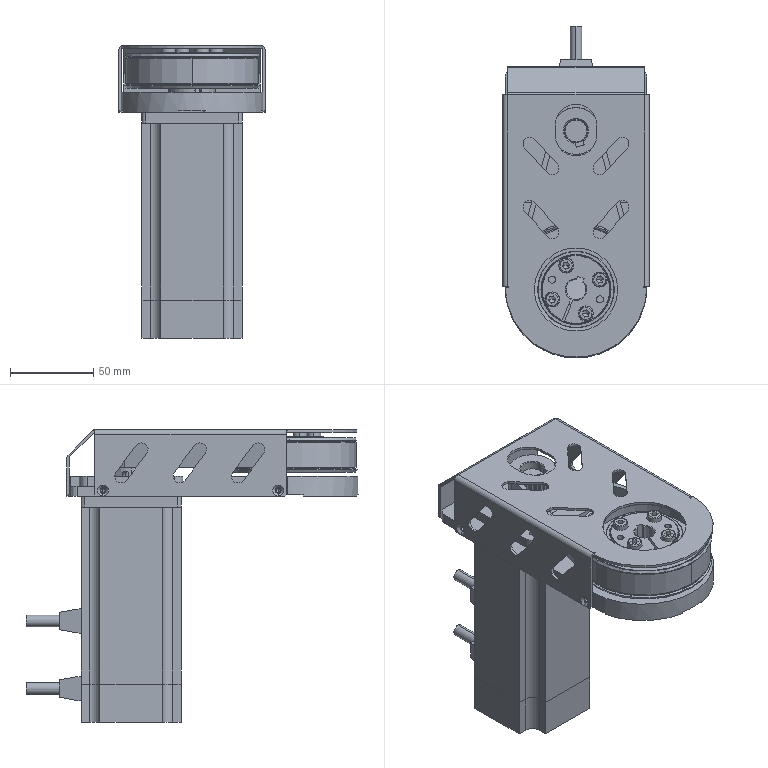Part | STEP file | Copy of CZ006-400W side connector 3:1(K60)^K50A-1H20-S(equation-driven)-L | 18 solids | 1174 faces | box 88 x 199.001 x 175.5 mm | volume 719497 mm3 | cylinder 784 | plane 262 | cone 110 | spline 18 | commonest cylinder face diameters 0.6 x269 1.82 x161 76.62 x82 8 x31 25.2 x28 5.5 x24